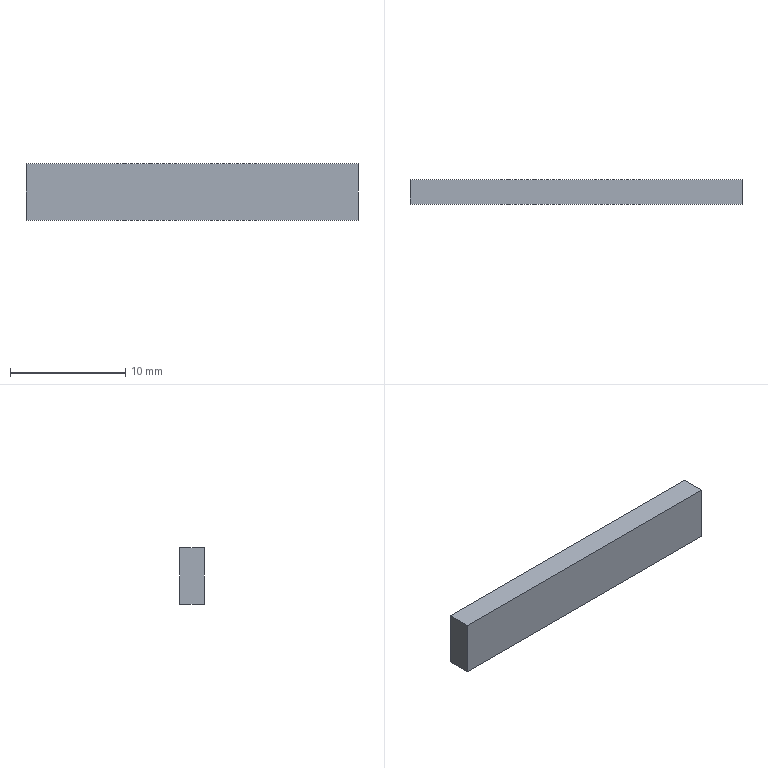Part | SolidWorks | features BaseBody 1 | 1 solid | 6 faces | box 28.83 x 2.1 x 4.91 mm | volume 297.266 mm3 | plane 6
STEP:
#1=CARTESIAN_POINT('',(14.415,0.,4.91));
#2=VERTEX_POINT('',#1);
#3=CARTESIAN_POINT('',(14.415,0.,0.));
#4=VERTEX_POINT('',#3);
#5=CARTESIAN_POINT('',(14.415,0.,0.));
#6=DIRECTION('',(0.,0.,-1.));
#7=VECTOR('',#6,1000.);
#8=LINE('',#5,#7);
#9=EDGE_CURVE('',#2,#4,#8,.T.);
#10=ORIENTED_EDGE('',*,*,#9,.F.);
#11=CARTESIAN_POINT('',(-14.415,0.,4.91));
#12=VERTEX_POINT('',#11);
#13=CARTESIAN_POINT('',(0.,0.,4.91));
#14=DIRECTION('',(1.,0.,0.));
#15=VECTOR('',#14,1000.);
#16=LINE('',#13,#15);
#17=EDGE_CURVE('',#12,#2,#16,.T.);
#18=ORIENTED_EDGE('',*,*,#17,.F.);
#19=CARTESIAN_POINT('',(-14.415,0.,0.));
#20=VERTEX_POINT('',#19);
#21=CARTESIAN_POINT('',(-14.415,0.,0.));
#22=DIRECTION('',(0.,0.,1.));
#23=VECTOR('',#22,1000.);
#24=LINE('',#21,#23);
#25=EDGE_CURVE('',#20,#12,#24,.T.);
#26=ORIENTED_EDGE('',*,*,#25,.F.);
#27=CARTESIAN_POINT('',(0.,0.,0.));
#28=DIRECTION('',(-1.,0.,0.));
#29=VECTOR('',#28,1000.);
#30=LINE('',#27,#29);
#31=EDGE_CURVE('',#4,#20,#30,.T.);
#32=ORIENTED_EDGE('',*,*,#31,.F.);
#33=EDGE_LOOP('',(#10,#18,#26,#32));
#34=FACE_OUTER_BOUND('',#33,.T.);
#35=CARTESIAN_POINT('',(0.,0.,0.));
#36=DIRECTION('',(0.,1.,0.));
#37=DIRECTION('',(0.,0.,1.));
#38=AXIS2_PLACEMENT_3D('',#35,#36,#37);
#39=PLANE('',#38);
#40=ADVANCED_FACE('',(#34),#39,.F.);
#41=CARTESIAN_POINT('',(14.415,2.1,0.));
#42=VERTEX_POINT('',#41);
#43=CARTESIAN_POINT('',(14.415,0.,0.));
#44=DIRECTION('',(0.,-1.,0.));
#45=VECTOR('',#44,1000.);
#46=LINE('',#43,#45);
#47=EDGE_CURVE('',#42,#4,#46,.T.);
#48=ORIENTED_EDGE('',*,*,#47,.T.);
#49=ORIENTED_EDGE('',*,*,#31,.T.);
#50=CARTESIAN_POINT('',(-14.415,2.1,0.));
#51=VERTEX_POINT('',#50);
#52=CARTESIAN_POINT('',(-14.415,0.,0.));
#53=DIRECTION('',(0.,1.,0.));
#54=VECTOR('',#53,1000.);
#55=LINE('',#52,#54);
#56=EDGE_CURVE('',#20,#51,#55,.T.);
#57=ORIENTED_EDGE('',*,*,#56,.T.);
#58=CARTESIAN_POINT('',(14.415,2.1,0.));
#59=DIRECTION('',(1.,0.,0.));
#60=VECTOR('',#59,1000.);
#61=LINE('',#58,#60);
#62=EDGE_CURVE('',#51,#42,#61,.T.);
#63=ORIENTED_EDGE('',*,*,#62,.T.);
#64=EDGE_LOOP('',(#48,#49,#57,#63));
#65=FACE_OUTER_BOUND('',#64,.T.);
#66=CARTESIAN_POINT('',(14.415,0.,0.));
#67=DIRECTION('',(0.,0.,-1.));
#68=DIRECTION('',(-1.,0.,0.));
#69=AXIS2_PLACEMENT_3D('',#66,#67,#68);
#70=PLANE('',#69);
#71=ADVANCED_FACE('',(#65),#70,.T.);
#72=CARTESIAN_POINT('',(14.415,2.1,4.91));
#73=VERTEX_POINT('',#72);
#74=CARTESIAN_POINT('',(14.415,0.,4.91));
#75=DIRECTION('',(0.,-1.,0.));
#76=VECTOR('',#75,1000.);
#77=LINE('',#74,#76);
#78=EDGE_CURVE('',#73,#2,#77,.T.);
#79=ORIENTED_EDGE('',*,*,#78,.T.);
#80=ORIENTED_EDGE('',*,*,#9,.T.);
#81=ORIENTED_EDGE('',*,*,#47,.F.);
#82=CARTESIAN_POINT('',(14.415,2.1,4.91));
#83=DIRECTION('',(0.,0.,1.));
#84=VECTOR('',#83,1000.);
#85=LINE('',#82,#84);
#86=EDGE_CURVE('',#42,#73,#85,.T.);
#87=ORIENTED_EDGE('',*,*,#86,.T.);
#88=EDGE_LOOP('',(#79,#80,#81,#87));
#89=FACE_OUTER_BOUND('',#88,.T.);
#90=CARTESIAN_POINT('',(14.415,0.,4.91));
#91=DIRECTION('',(1.,0.,0.));
#92=DIRECTION('',(0.,0.,-1.));
#93=AXIS2_PLACEMENT_3D('',#90,#91,#92);
#94=PLANE('',#93);
#95=ADVANCED_FACE('',(#89),#94,.T.);
#96=CARTESIAN_POINT('',(-14.415,2.1,4.91));
#97=VERTEX_POINT('',#96);
#98=CARTESIAN_POINT('',(-14.415,0.,4.91));
#99=DIRECTION('',(0.,-1.,0.));
#100=VECTOR('',#99,1000.);
#101=LINE('',#98,#100);
#102=EDGE_CURVE('',#97,#12,#101,.T.);
#103=ORIENTED_EDGE('',*,*,#102,.T.);
#104=ORIENTED_EDGE('',*,*,#17,.T.);
#105=ORIENTED_EDGE('',*,*,#78,.F.);
#106=CARTESIAN_POINT('',(-14.415,2.1,4.91));
#107=DIRECTION('',(-1.,0.,0.));
#108=VECTOR('',#107,1000.);
#109=LINE('',#106,#108);
#110=EDGE_CURVE('',#73,#97,#109,.T.);
#111=ORIENTED_EDGE('',*,*,#110,.T.);
#112=EDGE_LOOP('',(#103,#104,#105,#111));
#113=FACE_OUTER_BOUND('',#112,.T.);
#114=CARTESIAN_POINT('',(-14.415,0.,4.91));
#115=DIRECTION('',(0.,0.,1.));
#116=DIRECTION('',(1.,0.,0.));
#117=AXIS2_PLACEMENT_3D('',#114,#115,#116);
#118=PLANE('',#117);
#119=ADVANCED_FACE('',(#113),#118,.T.);
#120=ORIENTED_EDGE('',*,*,#56,.F.);
#121=ORIENTED_EDGE('',*,*,#25,.T.);
#122=ORIENTED_EDGE('',*,*,#102,.F.);
#123=CARTESIAN_POINT('',(-14.415,2.1,0.));
#124=DIRECTION('',(0.,0.,-1.));
#125=VECTOR('',#124,1000.);
#126=LINE('',#123,#125);
#127=EDGE_CURVE('',#97,#51,#126,.T.);
#128=ORIENTED_EDGE('',*,*,#127,.T.);
#129=EDGE_LOOP('',(#120,#121,#122,#128));
#130=FACE_OUTER_BOUND('',#129,.T.);
#131=CARTESIAN_POINT('',(-14.415,0.,0.));
#132=DIRECTION('',(-1.,0.,0.));
#133=DIRECTION('',(0.,0.,1.));
#134=AXIS2_PLACEMENT_3D('',#131,#132,#133);
#135=PLANE('',#134);
#136=ADVANCED_FACE('',(#130),#135,.T.);
#137=ORIENTED_EDGE('',*,*,#62,.F.);
#138=ORIENTED_EDGE('',*,*,#127,.F.);
#139=ORIENTED_EDGE('',*,*,#110,.F.);
#140=ORIENTED_EDGE('',*,*,#86,.F.);
#141=EDGE_LOOP('',(#137,#138,#139,#140));
#142=FACE_OUTER_BOUND('',#141,.T.);
#143=CARTESIAN_POINT('',(0.,2.1,0.));
#144=DIRECTION('',(0.,1.,0.));
#145=DIRECTION('',(0.,0.,1.));
#146=AXIS2_PLACEMENT_3D('',#143,#144,#145);
#147=PLANE('',#146);
#148=ADVANCED_FACE('',(#142),#147,.T.);
#149=CLOSED_SHELL('',(#40,#71,#95,#119,#136,#148));
#150=MANIFOLD_SOLID_BREP('',#149);
#151=CARTESIAN_POINT('',(0.,0.,0.));
#152=DIRECTION('',(0.,0.,1.));
#153=DIRECTION('',(1.,0.,0.));
#154=AXIS2_PLACEMENT_3D('',#151,#152,#153);
#155=(LENGTH_UNIT()NAMED_UNIT(*)SI_UNIT(.MILLI.,.METRE.));
#156=UNCERTAINTY_MEASURE_WITH_UNIT(LENGTH_MEASURE(0.00001),#155,'','');
#157=(NAMED_UNIT(*)PLANE_ANGLE_UNIT()SI_UNIT($,.RADIAN.));
#158=(NAMED_UNIT(*)SI_UNIT($,.STERADIAN.)SOLID_ANGLE_UNIT());
#159=(GEOMETRIC_REPRESENTATION_CONTEXT(3)GLOBAL_UNCERTAINTY_ASSIGNED_CONTEXT((#156))GLOBAL_UNIT_ASSIGNED_CONTEXT((#155,#157,#158))REPRESENTATION_CONTEXT('',''));
#160=ADVANCED_BREP_SHAPE_REPRESENTATION('',(#150,#154),#159);